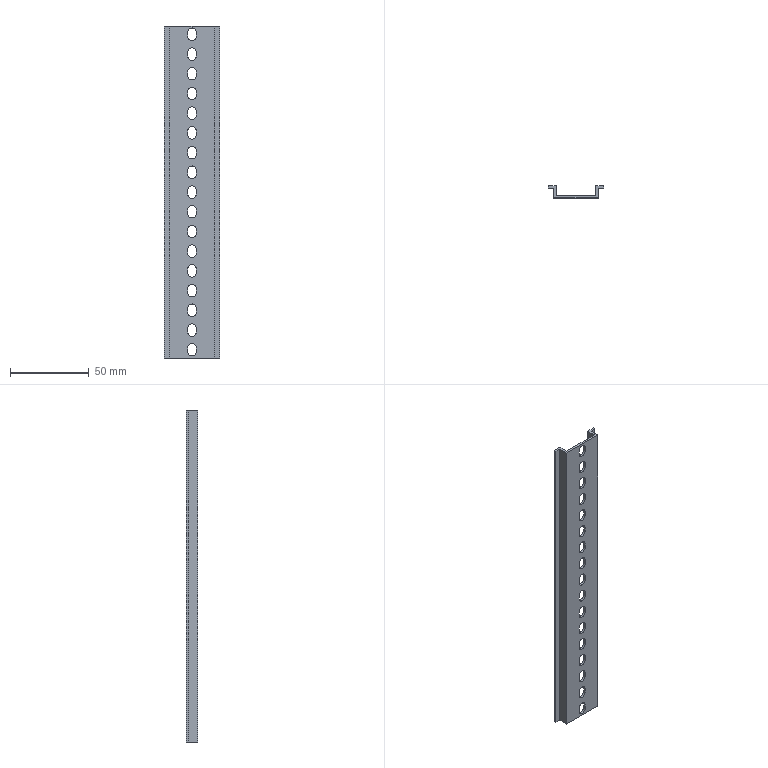Part | STEP file | SS5V1-16S3AD-08B-N1_AXT100-DR | 1 solid | 99 faces | box 35 x 7.5 x 210.5 mm | volume 13884 mm3 | cylinder 51 | plane 48 | commonest cylinder face diameters 5.5 x51